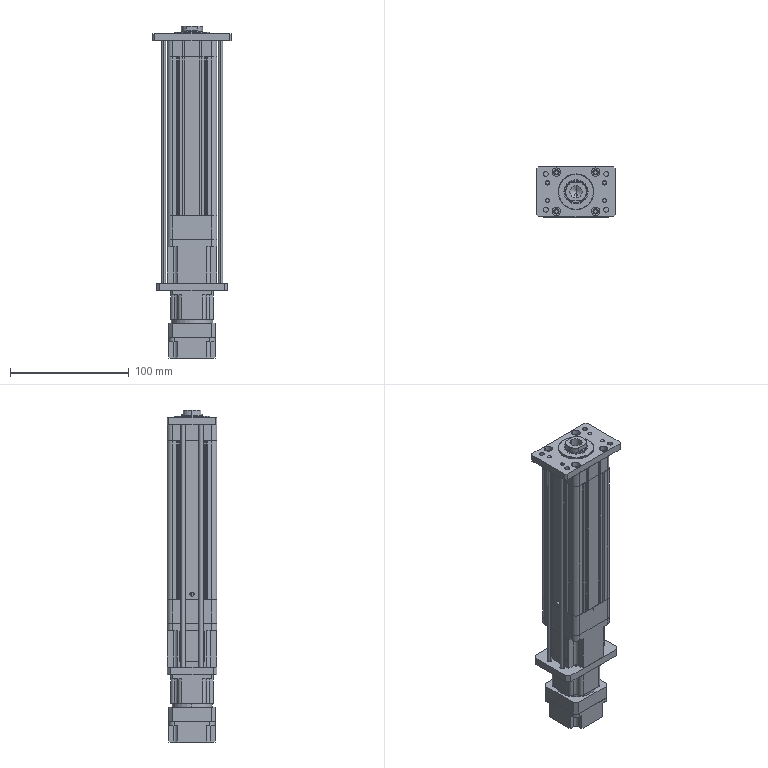Part | SolidWorks | features MBimport 1, MoveFace 1 | 16 solids | 787 faces | box 66 x 42 x 279.6 mm | volume 278895 mm3 | cylinder 376 | plane 330 | cone 81 | commonest cylinder face diameters 4.5 x32 3.6 x28 9 x28 4.2 x24 6 x22 1.5 x18